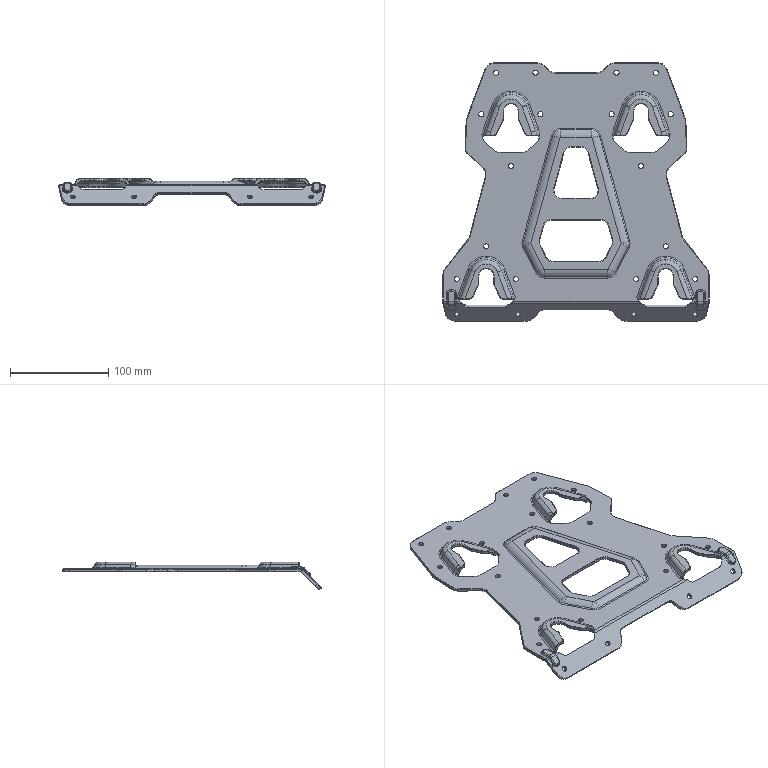Part | SolidWorks | features BaseBody 1 | 1 solid | 799 faces | box 270.301 x 262.271 x 28.314 mm | volume 151894 mm3 | plane 264 | cylinder 240 | cone 158 | torus 87 | spline 50 | commonest cylinder face diameters 2 x52 5.2 x40 10 x38 4 x36 20 x36 16 x10